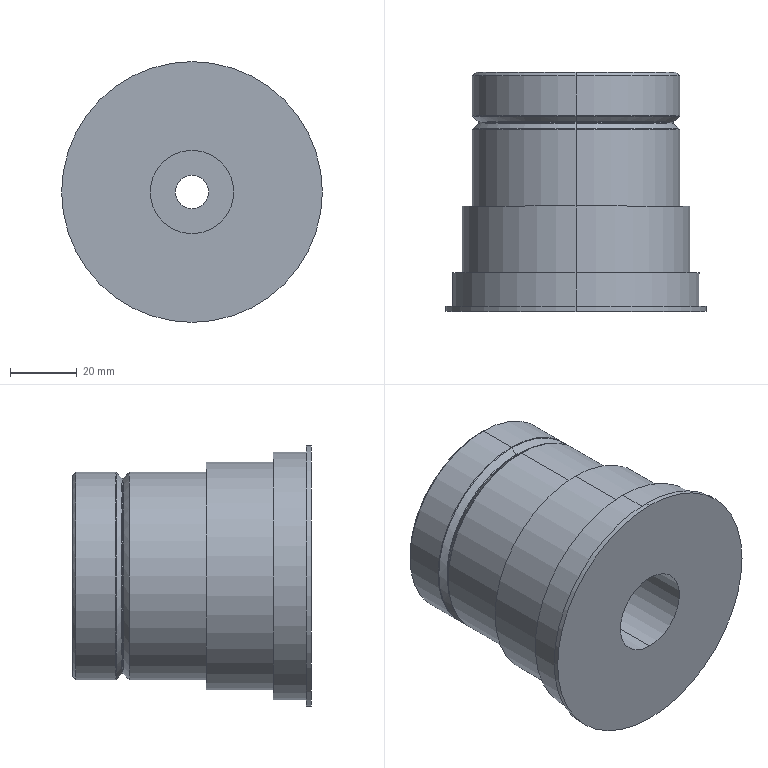Part | SolidWorks | features Chamfer 1, Revolution 1 | 1 solid | 34 faces | box 78 x 71.5 x 78 mm | volume 226793 mm3 | cylinder 14 | torus 8 | cone 6 | plane 6 | commonest cylinder face diameters 62 x4 10 x2 25 x2 68 x2 74 x2 78 x2
STEP:
#1=CARTESIAN_POINT('',(0.,56.288,-29.212));
#2=VERTEX_POINT('',#1);
#3=CARTESIAN_POINT('',(0.,56.5,-29.124));
#4=VERTEX_POINT('',#3);
#5=CARTESIAN_POINT('',(0.,56.5,-29.424));
#6=DIRECTION('',(-1.,0.,0.));
#7=DIRECTION('',(0.,0.,1.));
#8=AXIS2_PLACEMENT_3D('',#5,#6,#7);
#9=CIRCLE('',#8,0.3);
#10=EDGE_CURVE('',#2,#4,#9,.T.);
#11=ORIENTED_EDGE('',*,*,#10,.T.);
#12=CARTESIAN_POINT('',(0.,56.5,29.124));
#13=VERTEX_POINT('',#12);
#14=CARTESIAN_POINT('',(0.,56.5,0.));
#15=DIRECTION('',(0.,-1.,0.));
#16=DIRECTION('',(0.,0.,-1.));
#17=AXIS2_PLACEMENT_3D('',#14,#15,#16);
#18=CIRCLE('',#17,29.124);
#19=EDGE_CURVE('',#4,#13,#18,.T.);
#20=ORIENTED_EDGE('',*,*,#19,.T.);
#21=CARTESIAN_POINT('',(0.,56.288,29.212));
#22=VERTEX_POINT('',#21);
#23=CARTESIAN_POINT('',(0.,56.5,29.424));
#24=DIRECTION('',(1.,0.,0.));
#25=DIRECTION('',(0.,0.,-1.));
#26=AXIS2_PLACEMENT_3D('',#23,#24,#25);
#27=CIRCLE('',#26,0.3);
#28=EDGE_CURVE('',#22,#13,#27,.T.);
#29=ORIENTED_EDGE('',*,*,#28,.F.);
#30=CARTESIAN_POINT('',(0.,56.288,0.));
#31=DIRECTION('',(0.,-1.,0.));
#32=DIRECTION('',(0.,0.,-1.));
#33=AXIS2_PLACEMENT_3D('',#30,#31,#32);
#34=CIRCLE('',#33,29.212);
#35=EDGE_CURVE('',#2,#22,#34,.T.);
#36=ORIENTED_EDGE('',*,*,#35,.F.);
#37=EDGE_LOOP('',(#11,#20,#29,#36));
#38=FACE_OUTER_BOUND('',#37,.T.);
#39=CARTESIAN_POINT('',(0.,56.5,0.));
#40=DIRECTION('',(0.,-1.,0.));
#41=DIRECTION('',(0.,0.,-1.));
#42=AXIS2_PLACEMENT_3D('',#39,#40,#41);
#43=TOROIDAL_SURFACE('',#42,29.424,0.3);
#44=ADVANCED_FACE('',(#38),#43,.F.);
#45=ORIENTED_EDGE('',*,*,#28,.T.);
#46=CARTESIAN_POINT('',(0.,56.5,0.));
#47=DIRECTION('',(0.,-1.,0.));
#48=DIRECTION('',(0.,0.,-1.));
#49=AXIS2_PLACEMENT_3D('',#46,#47,#48);
#50=CIRCLE('',#49,29.124);
#51=EDGE_CURVE('',#13,#4,#50,.T.);
#52=ORIENTED_EDGE('',*,*,#51,.T.);
#53=ORIENTED_EDGE('',*,*,#10,.F.);
#54=CARTESIAN_POINT('',(0.,56.288,0.));
#55=DIRECTION('',(0.,-1.,0.));
#56=DIRECTION('',(0.,0.,-1.));
#57=AXIS2_PLACEMENT_3D('',#54,#55,#56);
#58=CIRCLE('',#57,29.212);
#59=EDGE_CURVE('',#22,#2,#58,.T.);
#60=ORIENTED_EDGE('',*,*,#59,.F.);
#61=EDGE_LOOP('',(#45,#52,#53,#60));
#62=FACE_OUTER_BOUND('',#61,.T.);
#63=CARTESIAN_POINT('',(0.,56.5,0.));
#64=DIRECTION('',(0.,-1.,0.));
#65=DIRECTION('',(0.,0.,-1.));
#66=AXIS2_PLACEMENT_3D('',#63,#64,#65);
#67=TOROIDAL_SURFACE('',#66,29.424,0.3);
#68=ADVANCED_FACE('',(#62),#67,.F.);
#69=CARTESIAN_POINT('',(0.,71.5,30.));
#70=VERTEX_POINT('',#69);
#71=CARTESIAN_POINT('',(0.,71.5,-30.));
#72=VERTEX_POINT('',#71);
#73=CARTESIAN_POINT('',(0.,71.5,0.));
#74=DIRECTION('',(0.,1.,0.));
#75=DIRECTION('',(0.,0.,-1.));
#76=AXIS2_PLACEMENT_3D('',#73,#74,#75);
#77=CIRCLE('',#76,30.);
#78=EDGE_CURVE('',#70,#72,#77,.T.);
#79=ORIENTED_EDGE('',*,*,#78,.F.);
#80=CARTESIAN_POINT('',(0.,70.5,31.));
#81=VERTEX_POINT('',#80);
#82=CARTESIAN_POINT('',(0.,70.5,31.));
#83=DIRECTION('',(0.,-0.7071,0.7071));
#84=VECTOR('',#83,1000.);
#85=LINE('',#82,#84);
#86=EDGE_CURVE('',#70,#81,#85,.T.);
#87=ORIENTED_EDGE('',*,*,#86,.T.);
#88=CARTESIAN_POINT('',(0.,70.5,-31.));
#89=VERTEX_POINT('',#88);
#90=CARTESIAN_POINT('',(0.,70.5,0.));
#91=DIRECTION('',(0.,-1.,0.));
#92=DIRECTION('',(0.,0.,-1.));
#93=AXIS2_PLACEMENT_3D('',#90,#91,#92);
#94=CIRCLE('',#93,31.);
#95=EDGE_CURVE('',#89,#81,#94,.T.);
#96=ORIENTED_EDGE('',*,*,#95,.F.);
#97=CARTESIAN_POINT('',(0.,70.5,-31.));
#98=DIRECTION('',(0.,-0.7071,-0.7071));
#99=VECTOR('',#98,1000.);
#100=LINE('',#97,#99);
#101=EDGE_CURVE('',#72,#89,#100,.T.);
#102=ORIENTED_EDGE('',*,*,#101,.F.);
#103=EDGE_LOOP('',(#79,#87,#96,#102));
#104=FACE_OUTER_BOUND('',#103,.T.);
#105=CARTESIAN_POINT('',(0.,70.5,0.));
#106=DIRECTION('',(0.,-1.,0.));
#107=DIRECTION('',(0.,0.,-1.));
#108=AXIS2_PLACEMENT_3D('',#105,#106,#107);
#109=CONICAL_SURFACE('',#108,31.,0.7854);
#110=ADVANCED_FACE('',(#104),#109,.T.);
#111=ORIENTED_EDGE('',*,*,#95,.T.);
#112=CARTESIAN_POINT('',(0.,58.624,31.));
#113=VERTEX_POINT('',#112);
#114=CARTESIAN_POINT('',(0.,0.,31.));
#115=DIRECTION('',(0.,-1.,0.));
#116=VECTOR('',#115,1000.);
#117=LINE('',#114,#116);
#118=EDGE_CURVE('',#81,#113,#117,.T.);
#119=ORIENTED_EDGE('',*,*,#118,.T.);
#120=CARTESIAN_POINT('',(0.,58.624,-31.));
#121=VERTEX_POINT('',#120);
#122=CARTESIAN_POINT('',(0.,58.624,0.));
#123=DIRECTION('',(0.,-1.,0.));
#124=DIRECTION('',(0.,0.,-1.));
#125=AXIS2_PLACEMENT_3D('',#122,#123,#124);
#126=CIRCLE('',#125,31.);
#127=EDGE_CURVE('',#121,#113,#126,.T.);
#128=ORIENTED_EDGE('',*,*,#127,.F.);
#129=CARTESIAN_POINT('',(0.,0.,-31.));
#130=DIRECTION('',(0.,-1.,0.));
#131=VECTOR('',#130,1000.);
#132=LINE('',#129,#131);
#133=EDGE_CURVE('',#89,#121,#132,.T.);
#134=ORIENTED_EDGE('',*,*,#133,.F.);
#135=EDGE_LOOP('',(#111,#119,#128,#134));
#136=FACE_OUTER_BOUND('',#135,.T.);
#137=CARTESIAN_POINT('',(0.,0.,0.));
#138=DIRECTION('',(0.,-1.,0.));
#139=DIRECTION('',(0.,0.,-1.));
#140=AXIS2_PLACEMENT_3D('',#137,#138,#139);
#141=CYLINDRICAL_SURFACE('',#140,31.);
#142=ADVANCED_FACE('',(#136),#141,.T.);
#143=CARTESIAN_POINT('',(0.,71.5,5.));
#144=VERTEX_POINT('',#143);
#145=CARTESIAN_POINT('',(0.,71.5,-5.));
#146=VERTEX_POINT('',#145);
#147=CARTESIAN_POINT('',(0.,71.5,0.));
#148=DIRECTION('',(0.,-1.,0.));
#149=DIRECTION('',(0.,0.,-1.));
#150=AXIS2_PLACEMENT_3D('',#147,#148,#149);
#151=CIRCLE('',#150,5.);
#152=EDGE_CURVE('',#144,#146,#151,.T.);
#153=ORIENTED_EDGE('',*,*,#152,.F.);
#154=CARTESIAN_POINT('',(0.,25.,5.));
#155=VERTEX_POINT('',#154);
#156=CARTESIAN_POINT('',(0.,0.,5.));
#157=DIRECTION('',(0.,-1.,0.));
#158=VECTOR('',#157,1000.);
#159=LINE('',#156,#158);
#160=EDGE_CURVE('',#144,#155,#159,.T.);
#161=ORIENTED_EDGE('',*,*,#160,.T.);
#162=CARTESIAN_POINT('',(0.,25.,-5.));
#163=VERTEX_POINT('',#162);
#164=CARTESIAN_POINT('',(0.,25.,0.));
#165=DIRECTION('',(0.,-1.,0.));
#166=DIRECTION('',(0.,0.,-1.));
#167=AXIS2_PLACEMENT_3D('',#164,#165,#166);
#168=CIRCLE('',#167,5.);
#169=EDGE_CURVE('',#155,#163,#168,.T.);
#170=ORIENTED_EDGE('',*,*,#169,.T.);
#171=CARTESIAN_POINT('',(0.,0.,-5.));
#172=DIRECTION('',(0.,-1.,0.));
#173=VECTOR('',#172,1000.);
#174=LINE('',#171,#173);
#175=EDGE_CURVE('',#146,#163,#174,.T.);
#176=ORIENTED_EDGE('',*,*,#175,.F.);
#177=EDGE_LOOP('',(#153,#161,#170,#176));
#178=FACE_OUTER_BOUND('',#177,.T.);
#179=CARTESIAN_POINT('',(0.,0.,0.));
#180=DIRECTION('',(0.,-1.,0.));
#181=DIRECTION('',(0.,0.,-1.));
#182=AXIS2_PLACEMENT_3D('',#179,#180,#181);
#183=CYLINDRICAL_SURFACE('',#182,5.);
#184=ADVANCED_FACE('',(#178),#183,.F.);
#185=CARTESIAN_POINT('',(0.,25.,12.5));
#186=VERTEX_POINT('',#185);
#187=CARTESIAN_POINT('',(0.,25.,-12.5));
#188=VERTEX_POINT('',#187);
#189=CARTESIAN_POINT('',(0.,25.,0.));
#190=DIRECTION('',(0.,-1.,0.));
#191=DIRECTION('',(0.,0.,-1.));
#192=AXIS2_PLACEMENT_3D('',#189,#190,#191);
#193=CIRCLE('',#192,12.5);
#194=EDGE_CURVE('',#186,#188,#193,.T.);
#195=ORIENTED_EDGE('',*,*,#194,.F.);
#196=CARTESIAN_POINT('',(0.,0.,12.5));
#197=VERTEX_POINT('',#196);
#198=CARTESIAN_POINT('',(0.,0.,12.5));
#199=DIRECTION('',(0.,-1.,0.));
#200=VECTOR('',#199,1000.);
#201=LINE('',#198,#200);
#202=EDGE_CURVE('',#186,#197,#201,.T.);
#203=ORIENTED_EDGE('',*,*,#202,.T.);
#204=CARTESIAN_POINT('',(0.,0.,-12.5));
#205=VERTEX_POINT('',#204);
#206=CARTESIAN_POINT('',(0.,0.,0.));
#207=DIRECTION('',(0.,-1.,0.));
#208=DIRECTION('',(0.,0.,-1.));
#209=AXIS2_PLACEMENT_3D('',#206,#207,#208);
#210=CIRCLE('',#209,12.5);
#211=EDGE_CURVE('',#197,#205,#210,.T.);
#212=ORIENTED_EDGE('',*,*,#211,.T.);
#213=CARTESIAN_POINT('',(0.,0.,-12.5));
#214=DIRECTION('',(0.,-1.,0.));
#215=VECTOR('',#214,1000.);
#216=LINE('',#213,#215);
#217=EDGE_CURVE('',#188,#205,#216,.T.);
#218=ORIENTED_EDGE('',*,*,#217,.F.);
#219=EDGE_LOOP('',(#195,#203,#212,#218));
#220=FACE_OUTER_BOUND('',#219,.T.);
#221=CARTESIAN_POINT('',(0.,0.,0.));
#222=DIRECTION('',(0.,-1.,0.));
#223=DIRECTION('',(0.,0.,-1.));
#224=AXIS2_PLACEMENT_3D('',#221,#222,#223);
#225=CYLINDRICAL_SURFACE('',#224,12.5);
#226=ADVANCED_FACE('',(#220),#225,.F.);
#227=CARTESIAN_POINT('',(0.,1.5,-39.));
#228=VERTEX_POINT('',#227);
#229=CARTESIAN_POINT('',(0.,1.5,39.));
#230=VERTEX_POINT('',#229);
#231=CARTESIAN_POINT('',(0.,1.5,0.));
#232=DIRECTION('',(0.,-1.,0.));
#233=DIRECTION('',(0.,0.,-1.));
#234=AXIS2_PLACEMENT_3D('',#231,#232,#233);
#235=CIRCLE('',#234,39.);
#236=EDGE_CURVE('',#228,#230,#235,.T.);
#237=ORIENTED_EDGE('',*,*,#236,.T.);
#238=CARTESIAN_POINT('',(0.,0.,39.));
#239=VERTEX_POINT('',#238);
#240=CARTESIAN_POINT('',(0.,0.,39.));
#241=DIRECTION('',(0.,-1.,0.));
#242=VECTOR('',#241,1000.);
#243=LINE('',#240,#242);
#244=EDGE_CURVE('',#230,#239,#243,.T.);
#245=ORIENTED_EDGE('',*,*,#244,.T.);
#246=CARTESIAN_POINT('',(0.,0.,-39.));
#247=VERTEX_POINT('',#246);
#248=CARTESIAN_POINT('',(0.,0.,0.));
#249=DIRECTION('',(0.,-1.,0.));
#250=DIRECTION('',(0.,0.,-1.));
#251=AXIS2_PLACEMENT_3D('',#248,#249,#250);
#252=CIRCLE('',#251,39.);
#253=EDGE_CURVE('',#247,#239,#252,.T.);
#254=ORIENTED_EDGE('',*,*,#253,.F.);
#255=CARTESIAN_POINT('',(0.,0.,-39.));
#256=DIRECTION('',(0.,-1.,0.));
#257=VECTOR('',#256,1000.);
#258=LINE('',#255,#257);
#259=EDGE_CURVE('',#228,#247,#258,.T.);
#260=ORIENTED_EDGE('',*,*,#259,.F.);
#261=EDGE_LOOP('',(#237,#245,#254,#260));
#262=FACE_OUTER_BOUND('',#261,.T.);
#263=CARTESIAN_POINT('',(0.,0.,0.));
#264=DIRECTION('',(0.,-1.,0.));
#265=DIRECTION('',(0.,0.,-1.));
#266=AXIS2_PLACEMENT_3D('',#263,#264,#265);
#267=CYLINDRICAL_SURFACE('',#266,39.);
#268=ADVANCED_FACE('',(#262),#267,.T.);
#269=CARTESIAN_POINT('',(0.,11.5,-37.));
#270=VERTEX_POINT('',#269);
#271=CARTESIAN_POINT('',(0.,11.5,37.));
#272=VERTEX_POINT('',#271);
#273=CARTESIAN_POINT('',(0.,11.5,0.));
#274=DIRECTION('',(0.,-1.,0.));
#275=DIRECTION('',(0.,0.,-1.));
#276=AXIS2_PLACEMENT_3D('',#273,#274,#275);
#277=CIRCLE('',#276,37.);
#278=EDGE_CURVE('',#270,#272,#277,.T.);
#279=ORIENTED_EDGE('',*,*,#278,.T.);
#280=CARTESIAN_POINT('',(0.,1.5,37.));
#281=VERTEX_POINT('',#280);
#282=CARTESIAN_POINT('',(0.,0.,37.));
#283=DIRECTION('',(0.,-1.,0.));
#284=VECTOR('',#283,1000.);
#285=LINE('',#282,#284);
#286=EDGE_CURVE('',#272,#281,#285,.T.);
#287=ORIENTED_EDGE('',*,*,#286,.T.);
#288=CARTESIAN_POINT('',(0.,1.5,-37.));
#289=VERTEX_POINT('',#288);
#290=CARTESIAN_POINT('',(0.,1.5,0.));
#291=DIRECTION('',(0.,-1.,0.));
#292=DIRECTION('',(0.,0.,-1.));
#293=AXIS2_PLACEMENT_3D('',#290,#291,#292);
#294=CIRCLE('',#293,37.);
#295=EDGE_CURVE('',#289,#281,#294,.T.);
#296=ORIENTED_EDGE('',*,*,#295,.F.);
#297=CARTESIAN_POINT('',(0.,0.,-37.));
#298=DIRECTION('',(0.,-1.,0.));
#299=VECTOR('',#298,1000.);
#300=LINE('',#297,#299);
#301=EDGE_CURVE('',#270,#289,#300,.T.);
#302=ORIENTED_EDGE('',*,*,#301,.F.);
#303=EDGE_LOOP('',(#279,#287,#296,#302));
#304=FACE_OUTER_BOUND('',#303,.T.);
#305=CARTESIAN_POINT('',(0.,0.,0.));
#306=DIRECTION('',(0.,-1.,0.));
#307=DIRECTION('',(0.,0.,-1.));
#308=AXIS2_PLACEMENT_3D('',#305,#306,#307);
#309=CYLINDRICAL_SURFACE('',#308,37.);
#310=ADVANCED_FACE('',(#304),#309,.T.);
#311=CARTESIAN_POINT('',(0.,31.5,-34.));
#312=VERTEX_POINT('',#311);
#313=CARTESIAN_POINT('',(0.,31.5,34.));
#314=VERTEX_POINT('',#313);
#315=CARTESIAN_POINT('',(0.,31.5,0.));
#316=DIRECTION('',(0.,-1.,0.));
#317=DIRECTION('',(0.,0.,-1.));
#318=AXIS2_PLACEMENT_3D('',#315,#316,#317);
#319=CIRCLE('',#318,34.);
#320=EDGE_CURVE('',#312,#314,#319,.T.);
#321=ORIENTED_EDGE('',*,*,#320,.T.);
#322=CARTESIAN_POINT('',(0.,11.5,34.));
#323=VERTEX_POINT('',#322);
#324=CARTESIAN_POINT('',(0.,0.,34.));
#325=DIRECTION('',(0.,-1.,0.));
#326=VECTOR('',#325,1000.);
#327=LINE('',#324,#326);
#328=EDGE_CURVE('',#314,#323,#327,.T.);
#329=ORIENTED_EDGE('',*,*,#328,.T.);
#330=CARTESIAN_POINT('',(0.,11.5,-34.));
#331=VERTEX_POINT('',#330);
#332=CARTESIAN_POINT('',(0.,11.5,0.));
#333=DIRECTION('',(0.,-1.,0.));
#334=DIRECTION('',(0.,0.,-1.));
#335=AXIS2_PLACEMENT_3D('',#332,#333,#334);
#336=CIRCLE('',#335,34.);
#337=EDGE_CURVE('',#331,#323,#336,.T.);
#338=ORIENTED_EDGE('',*,*,#337,.F.);
#339=CARTESIAN_POINT('',(0.,0.,-34.));
#340=DIRECTION('',(0.,-1.,0.));
#341=VECTOR('',#340,1000.);
#342=LINE('',#339,#341);
#343=EDGE_CURVE('',#312,#331,#342,.T.);
#344=ORIENTED_EDGE('',*,*,#343,.F.);
#345=EDGE_LOOP('',(#321,#329,#338,#344));
#346=FACE_OUTER_BOUND('',#345,.T.);
#347=CARTESIAN_POINT('',(0.,0.,0.));
#348=DIRECTION('',(0.,-1.,0.));
#349=DIRECTION('',(0.,0.,-1.));
#350=AXIS2_PLACEMENT_3D('',#347,#348,#349);
#351=CYLINDRICAL_SURFACE('',#350,34.);
#352=ADVANCED_FACE('',(#346),#351,.T.);
#353=CARTESIAN_POINT('',(0.,54.376,-31.));
#354=VERTEX_POINT('',#353);
#355=CARTESIAN_POINT('',(0.,54.376,31.));
#356=VERTEX_POINT('',#355);
#357=CARTESIAN_POINT('',(0.,54.376,0.));
#358=DIRECTION('',(0.,-1.,0.));
#359=DIRECTION('',(0.,0.,-1.));
#360=AXIS2_PLACEMENT_3D('',#357,#358,#359);
#361=CIRCLE('',#360,31.);
#362=EDGE_CURVE('',#354,#356,#361,.T.);
#363=ORIENTED_EDGE('',*,*,#362,.T.);
#364=CARTESIAN_POINT('',(0.,31.5,31.));
#365=VERTEX_POINT('',#364);
#366=CARTESIAN_POINT('',(0.,0.,31.));
#367=DIRECTION('',(0.,-1.,0.));
#368=VECTOR('',#367,1000.);
#369=LINE('',#366,#368);
#370=EDGE_CURVE('',#356,#365,#369,.T.);
#371=ORIENTED_EDGE('',*,*,#370,.T.);
#372=CARTESIAN_POINT('',(0.,31.5,-31.));
#373=VERTEX_POINT('',#372);
#374=CARTESIAN_POINT('',(0.,31.5,0.));
#375=DIRECTION('',(0.,-1.,0.));
#376=DIRECTION('',(0.,0.,-1.));
#377=AXIS2_PLACEMENT_3D('',#374,#375,#376);
#378=CIRCLE('',#377,31.);
#379=EDGE_CURVE('',#373,#365,#378,.T.);
#380=ORIENTED_EDGE('',*,*,#379,.F.);
#381=CARTESIAN_POINT('',(0.,0.,-31.));
#382=DIRECTION('',(0.,-1.,0.));
#383=VECTOR('',#382,1000.);
#384=LINE('',#381,#383);
#385=EDGE_CURVE('',#354,#373,#384,.T.);
#386=ORIENTED_EDGE('',*,*,#385,.F.);
#387=EDGE_LOOP('',(#363,#371,#380,#386));
#388=FACE_OUTER_BOUND('',#387,.T.);
#389=CARTESIAN_POINT('',(0.,0.,0.));
#390=DIRECTION('',(0.,-1.,0.));
#391=DIRECTION('',(0.,0.,-1.));
#392=AXIS2_PLACEMENT_3D('',#389,#390,#391);
#393=CYLINDRICAL_SURFACE('',#392,31.);
#394=ADVANCED_FACE('',(#388),#393,.T.);
#395=CARTESIAN_POINT('',(0.,54.588,-30.912));
#396=VERTEX_POINT('',#395);
#397=CARTESIAN_POINT('',(0.,54.588,30.912));
#398=VERTEX_POINT('',#397);
#399=CARTESIAN_POINT('',(0.,54.588,0.));
#400=DIRECTION('',(0.,-1.,0.));
#401=DIRECTION('',(0.,0.,-1.));
#402=AXIS2_PLACEMENT_3D('',#399,#400,#401);
#403=CIRCLE('',#402,30.912);
#404=EDGE_CURVE('',#396,#398,#403,.T.);
#405=ORIENTED_EDGE('',*,*,#404,.T.);
#406=CARTESIAN_POINT('',(0.,54.376,30.7));
#407=DIRECTION('',(1.,0.,0.));
#408=DIRECTION('',(0.,0.,-1.));
#409=AXIS2_PLACEMENT_3D('',#406,#407,#408);
#410=CIRCLE('',#409,0.3);
#411=EDGE_CURVE('',#398,#356,#410,.T.);
#412=ORIENTED_EDGE('',*,*,#411,.T.);
#413=ORIENTED_EDGE('',*,*,#362,.F.);
#414=CARTESIAN_POINT('',(0.,54.376,-30.7));
#415=DIRECTION('',(-1.,0.,0.));
#416=DIRECTION('',(0.,0.,1.));
#417=AXIS2_PLACEMENT_3D('',#414,#415,#416);
#418=CIRCLE('',#417,0.3);
#419=EDGE_CURVE('',#396,#354,#418,.T.);
#420=ORIENTED_EDGE('',*,*,#419,.F.);
#421=EDGE_LOOP('',(#405,#412,#413,#420));
#422=FACE_OUTER_BOUND('',#421,.T.);
#423=CARTESIAN_POINT('',(0.,54.376,0.));
#424=DIRECTION('',(0.,-1.,0.));
#425=DIRECTION('',(0.,0.,-1.));
#426=AXIS2_PLACEMENT_3D('',#423,#424,#425);
#427=TOROIDAL_SURFACE('',#426,30.7,0.3);
#428=ADVANCED_FACE('',(#422),#427,.T.);
#429=ORIENTED_EDGE('',*,*,#35,.T.);
#430=CARTESIAN_POINT('',(0.,56.288,29.212));
#431=DIRECTION('',(0.,-0.7071,0.7071));
#432=VECTOR('',#431,1000.);
#433=LINE('',#430,#432);
#434=EDGE_CURVE('',#22,#398,#433,.T.);
#435=ORIENTED_EDGE('',*,*,#434,.T.);
#436=ORIENTED_EDGE('',*,*,#404,.F.);
#437=CARTESIAN_POINT('',(0.,56.288,-29.212));
#438=DIRECTION('',(0.,-0.7071,-0.7071));
#439=VECTOR('',#438,1000.);
#440=LINE('',#437,#439);
#441=EDGE_CURVE('',#2,#396,#440,.T.);
#442=ORIENTED_EDGE('',*,*,#441,.F.);
#443=EDGE_LOOP('',(#429,#435,#436,#442));
#444=FACE_OUTER_BOUND('',#443,.T.);
#445=CARTESIAN_POINT('',(0.,56.288,0.));
#446=DIRECTION('',(0.,-1.,0.));
#447=DIRECTION('',(0.,0.,-1.));
#448=AXIS2_PLACEMENT_3D('',#445,#446,#447);
#449=CONICAL_SURFACE('',#448,29.212,0.7854);
#450=ADVANCED_FACE('',(#444),#449,.T.);
#451=ORIENTED_EDGE('',*,*,#51,.F.);
#452=CARTESIAN_POINT('',(0.,56.712,29.212));
#453=VERTEX_POINT('',#452);
#454=CARTESIAN_POINT('',(0.,56.5,29.424));
#455=DIRECTION('',(1.,0.,0.));
#456=DIRECTION('',(0.,0.,-1.));
#457=AXIS2_PLACEMENT_3D('',#454,#455,#456);
#458=CIRCLE('',#457,0.3);
#459=EDGE_CURVE('',#13,#453,#458,.T.);
#460=ORIENTED_EDGE('',*,*,#459,.T.);
#461=CARTESIAN_POINT('',(0.,56.712,-29.212));
#462=VERTEX_POINT('',#461);
#463=CARTESIAN_POINT('',(0.,56.712,0.));
#464=DIRECTION('',(0.,-1.,0.));
#465=DIRECTION('',(0.,0.,-1.));
#466=AXIS2_PLACEMENT_3D('',#463,#464,#465);
#467=CIRCLE('',#466,29.212);
#468=EDGE_CURVE('',#453,#462,#467,.T.);
#469=ORIENTED_EDGE('',*,*,#468,.T.);
#470=CARTESIAN_POINT('',(0.,56.5,-29.424));
#471=DIRECTION('',(-1.,0.,0.));
#472=DIRECTION('',(0.,0.,1.));
#473=AXIS2_PLACEMENT_3D('',#470,#471,#472);
#474=CIRCLE('',#473,0.3);
#475=EDGE_CURVE('',#4,#462,#474,.T.);
#476=ORIENTED_EDGE('',*,*,#475,.F.);
#477=EDGE_LOOP('',(#451,#460,#469,#476));
#478=FACE_OUTER_BOUND('',#477,.T.);
#479=CARTESIAN_POINT('',(0.,56.5,0.));
#480=DIRECTION('',(0.,-1.,0.));
#481=DIRECTION('',(0.,0.,-1.));
#482=AXIS2_PLACEMENT_3D('',#479,#480,#481);
#483=TOROIDAL_SURFACE('',#482,29.424,0.3);
#484=ADVANCED_FACE('',(#478),#483,.F.);
#485=CARTESIAN_POINT('',(0.,56.712,0.));
#486=DIRECTION('',(0.,-1.,0.));
#487=DIRECTION('',(0.,0.,-1.));
#488=AXIS2_PLACEMENT_3D('',#485,#486,#487);
#489=CIRCLE('',#488,29.212);
#490=EDGE_CURVE('',#462,#453,#489,.T.);
#491=ORIENTED_EDGE('',*,*,#490,.F.);
#492=CARTESIAN_POINT('',(0.,58.412,-30.912));
#493=VERTEX_POINT('',#492);
#494=CARTESIAN_POINT('',(0.,58.412,-30.912));
#495=DIRECTION('',(0.,0.7071,-0.7071));
#496=VECTOR('',#495,1000.);
#497=LINE('',#494,#496);
#498=EDGE_CURVE('',#462,#493,#497,.T.);
#499=ORIENTED_EDGE('',*,*,#498,.T.);
#500=CARTESIAN_POINT('',(0.,58.412,30.912));
#501=VERTEX_POINT('',#500);
#502=CARTESIAN_POINT('',(0.,58.412,0.));
#503=DIRECTION('',(0.,-1.,0.));
#504=DIRECTION('',(0.,0.,-1.));
#505=AXIS2_PLACEMENT_3D('',#502,#503,#504);
#506=CIRCLE('',#505,30.912);
#507=EDGE_CURVE('',#493,#501,#506,.T.);
#508=ORIENTED_EDGE('',*,*,#507,.T.);
#509=CARTESIAN_POINT('',(0.,58.412,30.912));
#510=DIRECTION('',(0.,0.7071,0.7071));
#511=VECTOR('',#510,1000.);
#512=LINE('',#509,#511);
#513=EDGE_CURVE('',#453,#501,#512,.T.);
#514=ORIENTED_EDGE('',*,*,#513,.F.);
#515=EDGE_LOOP('',(#491,#499,#508,#514));
#516=FACE_OUTER_BOUND('',#515,.T.);
#517=CARTESIAN_POINT('',(0.,58.412,0.));
#518=DIRECTION('',(0.,1.,0.));
#519=DIRECTION('',(0.,0.,1.));
#520=AXIS2_PLACEMENT_3D('',#517,#518,#519);
#521=CONICAL_SURFACE('',#520,30.912,0.7854);
#522=ADVANCED_FACE('',(#516),#521,.T.);
#523=ORIENTED_EDGE('',*,*,#127,.T.);
#524=CARTESIAN_POINT('',(0.,58.624,30.7));
#525=DIRECTION('',(1.,0.,0.));
#526=DIRECTION('',(0.,0.,-1.));
#527=AXIS2_PLACEMENT_3D('',#524,#525,#526);
#528=CIRCLE('',#527,0.3);
#529=EDGE_CURVE('',#113,#501,#528,.T.);
#530=ORIENTED_EDGE('',*,*,#529,.T.);
#531=ORIENTED_EDGE('',*,*,#507,.F.);
#532=CARTESIAN_POINT('',(0.,58.624,-30.7));
#533=DIRECTION('',(-1.,0.,0.));
#534=DIRECTION('',(0.,0.,1.));
#535=AXIS2_PLACEMENT_3D('',#532,#533,#534);
#536=CIRCLE('',#535,0.3);
#537=EDGE_CURVE('',#121,#493,#536,.T.);
#538=ORIENTED_EDGE('',*,*,#537,.F.);
#539=EDGE_LOOP('',(#523,#530,#531,#538));
#540=FACE_OUTER_BOUND('',#539,.T.);
#541=CARTESIAN_POINT('',(0.,58.624,0.));
#542=DIRECTION('',(0.,-1.,0.));
#543=DIRECTION('',(0.,0.,-1.));
#544=AXIS2_PLACEMENT_3D('',#541,#542,#543);
#545=TOROIDAL_SURFACE('',#544,30.7,0.3);
#546=ADVANCED_FACE('',(#540),#545,.T.);
#547=ORIENTED_EDGE('',*,*,#529,.F.);
#548=CARTESIAN_POINT('',(0.,58.624,0.));
#549=DIRECTION('',(0.,-1.,0.));
#550=DIRECTION('',(0.,0.,-1.));
#551=AXIS2_PLACEMENT_3D('',#548,#549,#550);
#552=CIRCLE('',#551,31.);
#553=EDGE_CURVE('',#113,#121,#552,.T.);
#554=ORIENTED_EDGE('',*,*,#553,.T.);
#555=ORIENTED_EDGE('',*,*,#537,.T.);
#556=CARTESIAN_POINT('',(0.,58.412,0.));
#557=DIRECTION('',(0.,-1.,0.));
#558=DIRECTION('',(0.,0.,-1.));
#559=AXIS2_PLACEMENT_3D('',#556,#557,#558);
#560=CIRCLE('',#559,30.912);
#561=EDGE_CURVE('',#501,#493,#560,.T.);
#562=ORIENTED_EDGE('',*,*,#561,.F.);
#563=EDGE_LOOP('',(#547,#554,#555,#562));
#564=FACE_OUTER_BOUND('',#563,.T.);
#565=CARTESIAN_POINT('',(0.,58.624,0.));
#566=DIRECTION('',(0.,-1.,0.));
#567=DIRECTION('',(0.,0.,-1.));
#568=AXIS2_PLACEMENT_3D('',#565,#566,#567);
#569=TOROIDAL_SURFACE('',#568,30.7,0.3);
#570=ADVANCED_FACE('',(#564),#569,.T.);
#571=ORIENTED_EDGE('',*,*,#498,.F.);
#572=ORIENTED_EDGE('',*,*,#468,.F.);
#573=ORIENTED_EDGE('',*,*,#513,.T.);
#574=ORIENTED_EDGE('',*,*,#561,.T.);
#575=EDGE_LOOP('',(#571,#572,#573,#574));
#576=FACE_OUTER_BOUND('',#575,.T.);
#577=CARTESIAN_POINT('',(0.,58.412,0.));
#578=DIRECTION('',(0.,1.,0.));
#579=DIRECTION('',(0.,0.,1.));
#580=AXIS2_PLACEMENT_3D('',#577,#578,#579);
#581=CONICAL_SURFACE('',#580,30.912,0.7854);
#582=ADVANCED_FACE('',(#576),#581,.T.);
#583=ORIENTED_EDGE('',*,*,#19,.F.);
#584=ORIENTED_EDGE('',*,*,#475,.T.);
#585=ORIENTED_EDGE('',*,*,#490,.T.);
#586=ORIENTED_EDGE('',*,*,#459,.F.);
#587=EDGE_LOOP('',(#583,#584,#585,#586));
#588=FACE_OUTER_BOUND('',#587,.T.);
#589=CARTESIAN_POINT('',(0.,56.5,0.));
#590=DIRECTION('',(0.,-1.,0.));
#591=DIRECTION('',(0.,0.,-1.));
#592=AXIS2_PLACEMENT_3D('',#589,#590,#591);
#593=TOROIDAL_SURFACE('',#592,29.424,0.3);
#594=ADVANCED_FACE('',(#588),#593,.F.);
#595=ORIENTED_EDGE('',*,*,#434,.F.);
#596=ORIENTED_EDGE('',*,*,#59,.T.);
#597=ORIENTED_EDGE('',*,*,#441,.T.);
#598=CARTESIAN_POINT('',(0.,54.588,0.));
#599=DIRECTION('',(0.,-1.,0.));
#600=DIRECTION('',(0.,0.,-1.));
#601=AXIS2_PLACEMENT_3D('',#598,#599,#600);
#602=CIRCLE('',#601,30.912);
#603=EDGE_CURVE('',#398,#396,#602,.T.);
#604=ORIENTED_EDGE('',*,*,#603,.F.);
#605=EDGE_LOOP('',(#595,#596,#597,#604));
#606=FACE_OUTER_BOUND('',#605,.T.);
#607=CARTESIAN_POINT('',(0.,56.288,0.));
#608=DIRECTION('',(0.,-1.,0.));
#609=DIRECTION('',(0.,0.,-1.));
#610=AXIS2_PLACEMENT_3D('',#607,#608,#609);
#611=CONICAL_SURFACE('',#610,29.212,0.7854);
#612=ADVANCED_FACE('',(#606),#611,.T.);
#613=ORIENTED_EDGE('',*,*,#411,.F.);
#614=ORIENTED_EDGE('',*,*,#603,.T.);
#615=ORIENTED_EDGE('',*,*,#419,.T.);
#616=CARTESIAN_POINT('',(0.,54.376,0.));
#617=DIRECTION('',(0.,-1.,0.));
#618=DIRECTION('',(0.,0.,-1.));
#619=AXIS2_PLACEMENT_3D('',#616,#617,#618);
#620=CIRCLE('',#619,31.);
#621=EDGE_CURVE('',#356,#354,#620,.T.);
#622=ORIENTED_EDGE('',*,*,#621,.F.);
#623=EDGE_LOOP('',(#613,#614,#615,#622));
#624=FACE_OUTER_BOUND('',#623,.T.);
#625=CARTESIAN_POINT('',(0.,54.376,0.));
#626=DIRECTION('',(0.,-1.,0.));
#627=DIRECTION('',(0.,0.,-1.));
#628=AXIS2_PLACEMENT_3D('',#625,#626,#627);
#629=TOROIDAL_SURFACE('',#628,30.7,0.3);
#630=ADVANCED_FACE('',(#624),#629,.T.);
#631=ORIENTED_EDGE('',*,*,#370,.F.);
#632=ORIENTED_EDGE('',*,*,#621,.T.);
#633=ORIENTED_EDGE('',*,*,#385,.T.);
#634=CARTESIAN_POINT('',(0.,31.5,0.));
#635=DIRECTION('',(0.,-1.,0.));
#636=DIRECTION('',(0.,0.,-1.));
#637=AXIS2_PLACEMENT_3D('',#634,#635,#636);
#638=CIRCLE('',#637,31.);
#639=EDGE_CURVE('',#365,#373,#638,.T.);
#640=ORIENTED_EDGE('',*,*,#639,.F.);
#641=EDGE_LOOP('',(#631,#632,#633,#640));
#642=FACE_OUTER_BOUND('',#641,.T.);
#643=CARTESIAN_POINT('',(0.,0.,0.));
#644=DIRECTION('',(0.,-1.,0.));
#645=DIRECTION('',(0.,0.,-1.));
#646=AXIS2_PLACEMENT_3D('',#643,#644,#645);
#647=CYLINDRICAL_SURFACE('',#646,31.);
#648=ADVANCED_FACE('',(#642),#647,.T.);
#649=ORIENTED_EDGE('',*,*,#320,.F.);
#650=CARTESIAN_POINT('',(0.,31.5,0.));
#651=DIRECTION('',(0.,-1.,0.));
#652=DIRECTION('',(0.,0.,-1.));
#653=AXIS2_PLACEMENT_3D('',#650,#651,#652);
#654=CIRCLE('',#653,34.);
#655=EDGE_CURVE('',#314,#312,#654,.T.);
#656=ORIENTED_EDGE('',*,*,#655,.F.);
#657=EDGE_LOOP('',(#649,#656));
#658=FACE_OUTER_BOUND('',#657,.T.);
#659=ORIENTED_EDGE('',*,*,#379,.T.);
#660=ORIENTED_EDGE('',*,*,#639,.T.);
#661=EDGE_LOOP('',(#659,#660));
#662=FACE_BOUND('',#661,.T.);
#663=CARTESIAN_POINT('',(-31.,31.5,0.));
#664=DIRECTION('',(0.,-1.,0.));
#665=DIRECTION('',(0.,0.,-1.));
#666=AXIS2_PLACEMENT_3D('',#663,#664,#665);
#667=PLANE('',#666);
#668=ADVANCED_FACE('',(#658,#662),#667,.F.);
#669=ORIENTED_EDGE('',*,*,#328,.F.);
#670=ORIENTED_EDGE('',*,*,#655,.T.);
#671=ORIENTED_EDGE('',*,*,#343,.T.);
#672=CARTESIAN_POINT('',(0.,11.5,0.));
#673=DIRECTION('',(0.,-1.,0.));
#674=DIRECTION('',(0.,0.,-1.));
#675=AXIS2_PLACEMENT_3D('',#672,#673,#674);
#676=CIRCLE('',#675,34.);
#677=EDGE_CURVE('',#323,#331,#676,.T.);
#678=ORIENTED_EDGE('',*,*,#677,.F.);
#679=EDGE_LOOP('',(#669,#670,#671,#678));
#680=FACE_OUTER_BOUND('',#679,.T.);
#681=CARTESIAN_POINT('',(0.,0.,0.));
#682=DIRECTION('',(0.,-1.,0.));
#683=DIRECTION('',(0.,0.,-1.));
#684=AXIS2_PLACEMENT_3D('',#681,#682,#683);
#685=CYLINDRICAL_SURFACE('',#684,34.);
#686=ADVANCED_FACE('',(#680),#685,.T.);
#687=ORIENTED_EDGE('',*,*,#278,.F.);
#688=CARTESIAN_POINT('',(0.,11.5,0.));
#689=DIRECTION('',(0.,-1.,0.));
#690=DIRECTION('',(0.,0.,-1.));
#691=AXIS2_PLACEMENT_3D('',#688,#689,#690);
#692=CIRCLE('',#691,37.);
#693=EDGE_CURVE('',#272,#270,#692,.T.);
#694=ORIENTED_EDGE('',*,*,#693,.F.);
#695=EDGE_LOOP('',(#687,#694));
#696=FACE_OUTER_BOUND('',#695,.T.);
#697=ORIENTED_EDGE('',*,*,#337,.T.);
#698=ORIENTED_EDGE('',*,*,#677,.T.);
#699=EDGE_LOOP('',(#697,#698));
#700=FACE_BOUND('',#699,.T.);
#701=CARTESIAN_POINT('',(-34.,11.5,0.));
#702=DIRECTION('',(0.,-1.,0.));
#703=DIRECTION('',(0.,0.,-1.));
#704=AXIS2_PLACEMENT_3D('',#701,#702,#703);
#705=PLANE('',#704);
#706=ADVANCED_FACE('',(#696,#700),#705,.F.);
#707=ORIENTED_EDGE('',*,*,#286,.F.);
#708=ORIENTED_EDGE('',*,*,#693,.T.);
#709=ORIENTED_EDGE('',*,*,#301,.T.);
#710=CARTESIAN_POINT('',(0.,1.5,0.));
#711=DIRECTION('',(0.,-1.,0.));
#712=DIRECTION('',(0.,0.,-1.));
#713=AXIS2_PLACEMENT_3D('',#710,#711,#712);
#714=CIRCLE('',#713,37.);
#715=EDGE_CURVE('',#281,#289,#714,.T.);
#716=ORIENTED_EDGE('',*,*,#715,.F.);
#717=EDGE_LOOP('',(#707,#708,#709,#716));
#718=FACE_OUTER_BOUND('',#717,.T.);
#719=CARTESIAN_POINT('',(0.,0.,0.));
#720=DIRECTION('',(0.,-1.,0.));
#721=DIRECTION('',(0.,0.,-1.));
#722=AXIS2_PLACEMENT_3D('',#719,#720,#721);
#723=CYLINDRICAL_SURFACE('',#722,37.);
#724=ADVANCED_FACE('',(#718),#723,.T.);
#725=ORIENTED_EDGE('',*,*,#236,.F.);
#726=CARTESIAN_POINT('',(0.,1.5,0.));
#727=DIRECTION('',(0.,-1.,0.));
#728=DIRECTION('',(0.,0.,-1.));
#729=AXIS2_PLACEMENT_3D('',#726,#727,#728);
#730=CIRCLE('',#729,39.);
#731=EDGE_CURVE('',#230,#228,#730,.T.);
#732=ORIENTED_EDGE('',*,*,#731,.F.);
#733=EDGE_LOOP('',(#725,#732));
#734=FACE_OUTER_BOUND('',#733,.T.);
#735=ORIENTED_EDGE('',*,*,#295,.T.);
#736=ORIENTED_EDGE('',*,*,#715,.T.);
#737=EDGE_LOOP('',(#735,#736));
#738=FACE_BOUND('',#737,.T.);
#739=CARTESIAN_POINT('',(-37.,1.5,0.));
#740=DIRECTION('',(0.,-1.,0.));
#741=DIRECTION('',(0.,0.,-1.));
#742=AXIS2_PLACEMENT_3D('',#739,#740,#741);
#743=PLANE('',#742);
#744=ADVANCED_FACE('',(#734,#738),#743,.F.);
#745=ORIENTED_EDGE('',*,*,#244,.F.);
#746=ORIENTED_EDGE('',*,*,#731,.T.);
#747=ORIENTED_EDGE('',*,*,#259,.T.);
#748=CARTESIAN_POINT('',(0.,0.,0.));
#749=DIRECTION('',(0.,-1.,0.));
#750=DIRECTION('',(0.,0.,-1.));
#751=AXIS2_PLACEMENT_3D('',#748,#749,#750);
#752=CIRCLE('',#751,39.);
#753=EDGE_CURVE('',#239,#247,#752,.T.);
#754=ORIENTED_EDGE('',*,*,#753,.F.);
#755=EDGE_LOOP('',(#745,#746,#747,#754));
#756=FACE_OUTER_BOUND('',#755,.T.);
#757=CARTESIAN_POINT('',(0.,0.,0.));
#758=DIRECTION('',(0.,-1.,0.));
#759=DIRECTION('',(0.,0.,-1.));
#760=AXIS2_PLACEMENT_3D('',#757,#758,#759);
#761=CYLINDRICAL_SURFACE('',#760,39.);
#762=ADVANCED_FACE('',(#756),#761,.T.);
#763=CARTESIAN_POINT('',(0.,0.,0.));
#764=DIRECTION('',(0.,-1.,0.));
#765=DIRECTION('',(0.,0.,-1.));
#766=AXIS2_PLACEMENT_3D('',#763,#764,#765);
#767=CIRCLE('',#766,12.5);
#768=EDGE_CURVE('',#205,#197,#767,.T.);
#769=ORIENTED_EDGE('',*,*,#768,.F.);
#770=ORIENTED_EDGE('',*,*,#211,.F.);
#771=EDGE_LOOP('',(#769,#770));
#772=FACE_BOUND('',#771,.T.);
#773=ORIENTED_EDGE('',*,*,#253,.T.);
#774=ORIENTED_EDGE('',*,*,#753,.T.);
#775=EDGE_LOOP('',(#773,#774));
#776=FACE_OUTER_BOUND('',#775,.T.);
#777=CARTESIAN_POINT('',(-39.,0.,0.));
#778=DIRECTION('',(0.,1.,0.));
#779=DIRECTION('',(0.,0.,1.));
#780=AXIS2_PLACEMENT_3D('',#777,#778,#779);
#781=PLANE('',#780);
#782=ADVANCED_FACE('',(#772,#776),#781,.F.);
#783=ORIENTED_EDGE('',*,*,#202,.F.);
#784=CARTESIAN_POINT('',(0.,25.,0.));
#785=DIRECTION('',(0.,-1.,0.));
#786=DIRECTION('',(0.,0.,-1.));
#787=AXIS2_PLACEMENT_3D('',#784,#785,#786);
#788=CIRCLE('',#787,12.5);
#789=EDGE_CURVE('',#188,#186,#788,.T.);
#790=ORIENTED_EDGE('',*,*,#789,.F.);
#791=ORIENTED_EDGE('',*,*,#217,.T.);
#792=ORIENTED_EDGE('',*,*,#768,.T.);
#793=EDGE_LOOP('',(#783,#790,#791,#792));
#794=FACE_OUTER_BOUND('',#793,.T.);
#795=CARTESIAN_POINT('',(0.,0.,0.));
#796=DIRECTION('',(0.,-1.,0.));
#797=DIRECTION('',(0.,0.,-1.));
#798=AXIS2_PLACEMENT_3D('',#795,#796,#797);
#799=CYLINDRICAL_SURFACE('',#798,12.5);
#800=ADVANCED_FACE('',(#794),#799,.F.);
#801=CARTESIAN_POINT('',(0.,25.,0.));
#802=DIRECTION('',(0.,-1.,0.));
#803=DIRECTION('',(0.,0.,-1.));
#804=AXIS2_PLACEMENT_3D('',#801,#802,#803);
#805=CIRCLE('',#804,5.);
#806=EDGE_CURVE('',#163,#155,#805,.T.);
#807=ORIENTED_EDGE('',*,*,#806,.F.);
#808=ORIENTED_EDGE('',*,*,#169,.F.);
#809=EDGE_LOOP('',(#807,#808));
#810=FACE_BOUND('',#809,.T.);
#811=ORIENTED_EDGE('',*,*,#789,.T.);
#812=ORIENTED_EDGE('',*,*,#194,.T.);
#813=EDGE_LOOP('',(#811,#812));
#814=FACE_OUTER_BOUND('',#813,.T.);
#815=CARTESIAN_POINT('',(-12.5,25.,0.));
#816=DIRECTION('',(0.,1.,0.));
#817=DIRECTION('',(0.,0.,1.));
#818=AXIS2_PLACEMENT_3D('',#815,#816,#817);
#819=PLANE('',#818);
#820=ADVANCED_FACE('',(#810,#814),#819,.F.);
#821=ORIENTED_EDGE('',*,*,#160,.F.);
#822=CARTESIAN_POINT('',(0.,71.5,0.));
#823=DIRECTION('',(0.,-1.,0.));
#824=DIRECTION('',(0.,0.,-1.));
#825=AXIS2_PLACEMENT_3D('',#822,#823,#824);
#826=CIRCLE('',#825,5.);
#827=EDGE_CURVE('',#146,#144,#826,.T.);
#828=ORIENTED_EDGE('',*,*,#827,.F.);
#829=ORIENTED_EDGE('',*,*,#175,.T.);
#830=ORIENTED_EDGE('',*,*,#806,.T.);
#831=EDGE_LOOP('',(#821,#828,#829,#830));
#832=FACE_OUTER_BOUND('',#831,.T.);
#833=CARTESIAN_POINT('',(0.,0.,0.));
#834=DIRECTION('',(0.,-1.,0.));
#835=DIRECTION('',(0.,0.,-1.));
#836=AXIS2_PLACEMENT_3D('',#833,#834,#835);
#837=CYLINDRICAL_SURFACE('',#836,5.);
#838=ADVANCED_FACE('',(#832),#837,.F.);
#839=CARTESIAN_POINT('',(0.,71.5,0.));
#840=DIRECTION('',(0.,1.,0.));
#841=DIRECTION('',(0.,0.,-1.));
#842=AXIS2_PLACEMENT_3D('',#839,#840,#841);
#843=CIRCLE('',#842,30.);
#844=EDGE_CURVE('',#72,#70,#843,.T.);
#845=ORIENTED_EDGE('',*,*,#844,.T.);
#846=ORIENTED_EDGE('',*,*,#78,.T.);
#847=EDGE_LOOP('',(#845,#846));
#848=FACE_OUTER_BOUND('',#847,.T.);
#849=ORIENTED_EDGE('',*,*,#827,.T.);
#850=ORIENTED_EDGE('',*,*,#152,.T.);
#851=EDGE_LOOP('',(#849,#850));
#852=FACE_BOUND('',#851,.T.);
#853=CARTESIAN_POINT('',(-5.,71.5,0.));
#854=DIRECTION('',(0.,-1.,0.));
#855=DIRECTION('',(0.,0.,-1.));
#856=AXIS2_PLACEMENT_3D('',#853,#854,#855);
#857=PLANE('',#856);
#858=ADVANCED_FACE('',(#848,#852),#857,.F.);
#859=ORIENTED_EDGE('',*,*,#118,.F.);
#860=CARTESIAN_POINT('',(0.,70.5,0.));
#861=DIRECTION('',(0.,-1.,0.));
#862=DIRECTION('',(0.,0.,-1.));
#863=AXIS2_PLACEMENT_3D('',#860,#861,#862);
#864=CIRCLE('',#863,31.);
#865=EDGE_CURVE('',#81,#89,#864,.T.);
#866=ORIENTED_EDGE('',*,*,#865,.T.);
#867=ORIENTED_EDGE('',*,*,#133,.T.);
#868=ORIENTED_EDGE('',*,*,#553,.F.);
#869=EDGE_LOOP('',(#859,#866,#867,#868));
#870=FACE_OUTER_BOUND('',#869,.T.);
#871=CARTESIAN_POINT('',(0.,0.,0.));
#872=DIRECTION('',(0.,-1.,0.));
#873=DIRECTION('',(0.,0.,-1.));
#874=AXIS2_PLACEMENT_3D('',#871,#872,#873);
#875=CYLINDRICAL_SURFACE('',#874,31.);
#876=ADVANCED_FACE('',(#870),#875,.T.);
#877=ORIENTED_EDGE('',*,*,#86,.F.);
#878=ORIENTED_EDGE('',*,*,#844,.F.);
#879=ORIENTED_EDGE('',*,*,#101,.T.);
#880=ORIENTED_EDGE('',*,*,#865,.F.);
#881=EDGE_LOOP('',(#877,#878,#879,#880));
#882=FACE_OUTER_BOUND('',#881,.T.);
#883=CARTESIAN_POINT('',(0.,70.5,0.));
#884=DIRECTION('',(0.,-1.,0.));
#885=DIRECTION('',(0.,0.,-1.));
#886=AXIS2_PLACEMENT_3D('',#883,#884,#885);
#887=CONICAL_SURFACE('',#886,31.,0.7854);
#888=ADVANCED_FACE('',(#882),#887,.T.);
#889=CLOSED_SHELL('',(#44,#68,#110,#142,#184,#226,#268,#310,#352,#394,#428,#450,#484,#522,#546,#570,#582,#594,#612,#630,#648,#668,#686,#706,#724,#744,#762,#782,#800,#820,#838,#858,#876,#888));
#890=MANIFOLD_SOLID_BREP('',#889);
#891=CARTESIAN_POINT('',(0.,0.,0.));
#892=DIRECTION('',(0.,0.,1.));
#893=DIRECTION('',(1.,0.,0.));
#894=AXIS2_PLACEMENT_3D('',#891,#892,#893);
#895=(LENGTH_UNIT()NAMED_UNIT(*)SI_UNIT(.MILLI.,.METRE.));
#896=UNCERTAINTY_MEASURE_WITH_UNIT(LENGTH_MEASURE(0.00001),#895,'','');
#897=(NAMED_UNIT(*)PLANE_ANGLE_UNIT()SI_UNIT($,.RADIAN.));
#898=(NAMED_UNIT(*)SI_UNIT($,.STERADIAN.)SOLID_ANGLE_UNIT());
#899=(GEOMETRIC_REPRESENTATION_CONTEXT(3)GLOBAL_UNCERTAINTY_ASSIGNED_CONTEXT((#896))GLOBAL_UNIT_ASSIGNED_CONTEXT((#895,#897,#898))REPRESENTATION_CONTEXT('',''));
#900=ADVANCED_BREP_SHAPE_REPRESENTATION('',(#890,#894),#899);